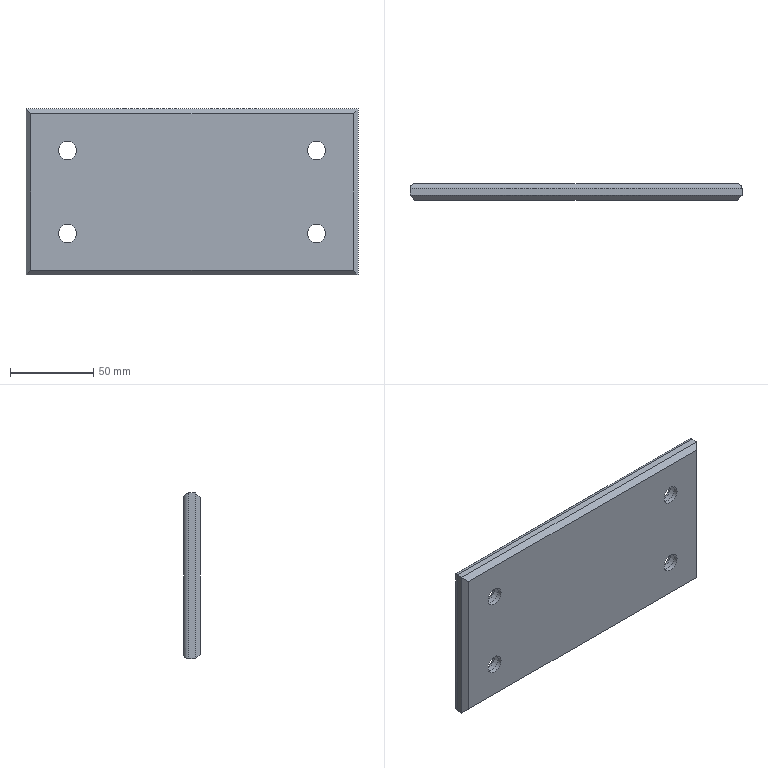Part | STEP file | lll_id4214_x_t | 1 solid | 166 faces | box 200 x 10 x 100 mm | volume 187810 mm3 | plane 109 | other 41 | cylinder 12 | torus 4 | commonest cylinder face diameters 6 x4 11 x4 17.5 x4